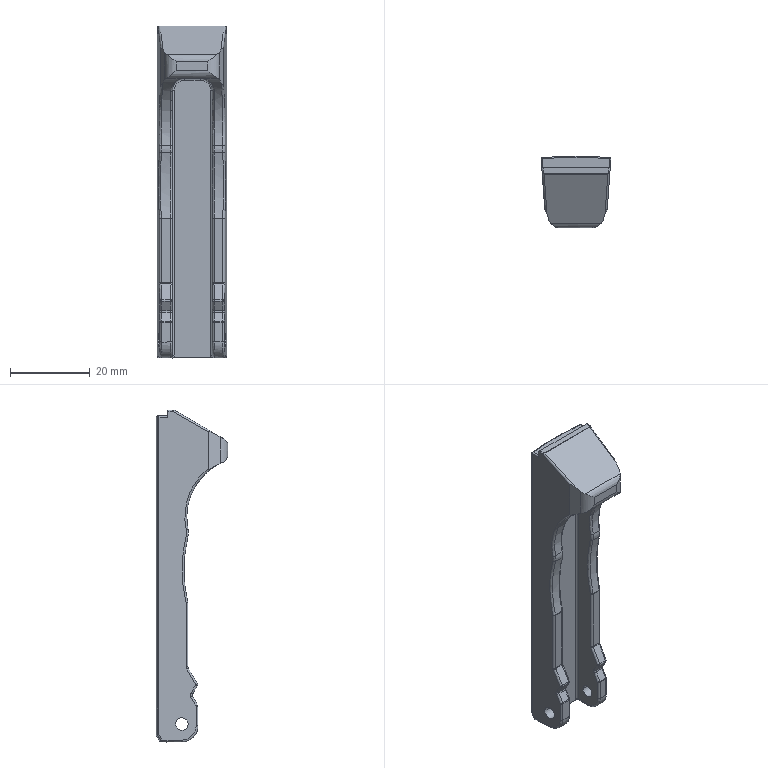Part | STEP file | _X2_751F4E45_X0_MS731-1_X2_8F_8 | 1 solid | 147 faces | box 17.395 x 18 x 83 mm | volume 8684 mm3 | cylinder 68 | plane 24 | torus 20 | spline 20 | sphere 14 | cone 1 | commonest cylinder face diameters 1 x40 0.6 x9 3.1 x4 6 x4 8 x4 4 x2